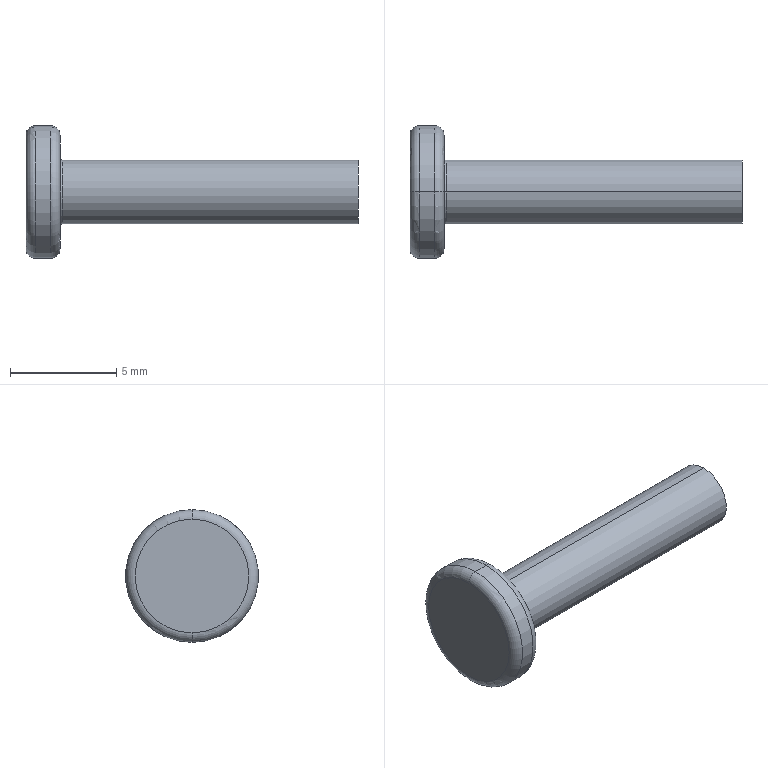Part | SolidWorks | features Revolution 1 | 1 solid | 13 faces | box 15.6 x 6.24 x 6.24 mm | volume 146.299 mm3 | torus 6 | cylinder 4 | plane 3 | commonest cylinder face diameters 3 x2 6.24 x2
STEP:
#1=CARTESIAN_POINT('',(0.4448,0.,3.12));
#2=VERTEX_POINT('',#1);
#3=CARTESIAN_POINT('',(0.4448,0.,-3.12));
#4=VERTEX_POINT('',#3);
#5=CARTESIAN_POINT('',(0.4448,0.,0.));
#6=DIRECTION('',(-1.,0.,0.));
#7=DIRECTION('',(0.,0.,1.));
#8=AXIS2_PLACEMENT_3D('',#5,#6,#7);
#9=CIRCLE('',#8,3.12);
#10=EDGE_CURVE('',#2,#4,#9,.T.);
#11=ORIENTED_EDGE('',*,*,#10,.T.);
#12=CARTESIAN_POINT('',(0.,0.,-2.675));
#13=VERTEX_POINT('',#12);
#14=CARTESIAN_POINT('',(0.4448,0.,-2.675));
#15=DIRECTION('',(0.,1.,0.));
#16=DIRECTION('',(0.,0.,1.));
#17=AXIS2_PLACEMENT_3D('',#14,#15,#16);
#18=CIRCLE('',#17,0.4448);
#19=EDGE_CURVE('',#4,#13,#18,.T.);
#20=ORIENTED_EDGE('',*,*,#19,.T.);
#21=CARTESIAN_POINT('',(0.,0.,2.675));
#22=VERTEX_POINT('',#21);
#23=CARTESIAN_POINT('',(0.,0.,0.));
#24=DIRECTION('',(-1.,0.,0.));
#25=DIRECTION('',(0.,0.,1.));
#26=AXIS2_PLACEMENT_3D('',#23,#24,#25);
#27=CIRCLE('',#26,2.675);
#28=EDGE_CURVE('',#22,#13,#27,.T.);
#29=ORIENTED_EDGE('',*,*,#28,.F.);
#30=CARTESIAN_POINT('',(0.4448,0.,2.675));
#31=DIRECTION('',(0.,-1.,0.));
#32=DIRECTION('',(0.,0.,-1.));
#33=AXIS2_PLACEMENT_3D('',#30,#31,#32);
#34=CIRCLE('',#33,0.4448);
#35=EDGE_CURVE('',#2,#22,#34,.T.);
#36=ORIENTED_EDGE('',*,*,#35,.F.);
#37=EDGE_LOOP('',(#11,#20,#29,#36));
#38=FACE_OUTER_BOUND('',#37,.T.);
#39=CARTESIAN_POINT('',(0.4448,0.,0.));
#40=DIRECTION('',(-1.,0.,0.));
#41=DIRECTION('',(0.,0.,1.));
#42=AXIS2_PLACEMENT_3D('',#39,#40,#41);
#43=TOROIDAL_SURFACE('',#42,2.675,0.4448);
#44=ADVANCED_FACE('',(#38),#43,.T.);
#45=CARTESIAN_POINT('',(1.155,0.,3.12));
#46=VERTEX_POINT('',#45);
#47=CARTESIAN_POINT('',(1.155,0.,-3.12));
#48=VERTEX_POINT('',#47);
#49=CARTESIAN_POINT('',(1.155,0.,0.));
#50=DIRECTION('',(-1.,0.,0.));
#51=DIRECTION('',(0.,0.,1.));
#52=AXIS2_PLACEMENT_3D('',#49,#50,#51);
#53=CIRCLE('',#52,3.12);
#54=EDGE_CURVE('',#46,#48,#53,.T.);
#55=ORIENTED_EDGE('',*,*,#54,.T.);
#56=CARTESIAN_POINT('',(0.,0.,-3.12));
#57=DIRECTION('',(-1.,0.,0.));
#58=VECTOR('',#57,1000.);
#59=LINE('',#56,#58);
#60=EDGE_CURVE('',#48,#4,#59,.T.);
#61=ORIENTED_EDGE('',*,*,#60,.T.);
#62=ORIENTED_EDGE('',*,*,#10,.F.);
#63=CARTESIAN_POINT('',(0.,0.,3.12));
#64=DIRECTION('',(-1.,0.,0.));
#65=VECTOR('',#64,1000.);
#66=LINE('',#63,#65);
#67=EDGE_CURVE('',#46,#2,#66,.T.);
#68=ORIENTED_EDGE('',*,*,#67,.F.);
#69=EDGE_LOOP('',(#55,#61,#62,#68));
#70=FACE_OUTER_BOUND('',#69,.T.);
#71=CARTESIAN_POINT('',(0.,0.,0.));
#72=DIRECTION('',(-1.,0.,0.));
#73=DIRECTION('',(0.,0.,1.));
#74=AXIS2_PLACEMENT_3D('',#71,#72,#73);
#75=CYLINDRICAL_SURFACE('',#74,3.12);
#76=ADVANCED_FACE('',(#70),#75,.T.);
#77=CARTESIAN_POINT('',(1.6,0.,2.675));
#78=VERTEX_POINT('',#77);
#79=CARTESIAN_POINT('',(1.6,0.,-2.675));
#80=VERTEX_POINT('',#79);
#81=CARTESIAN_POINT('',(1.6,0.,0.));
#82=DIRECTION('',(-1.,0.,0.));
#83=DIRECTION('',(0.,0.,1.));
#84=AXIS2_PLACEMENT_3D('',#81,#82,#83);
#85=CIRCLE('',#84,2.675);
#86=EDGE_CURVE('',#78,#80,#85,.T.);
#87=ORIENTED_EDGE('',*,*,#86,.T.);
#88=CARTESIAN_POINT('',(1.155,0.,-2.675));
#89=DIRECTION('',(0.,1.,0.));
#90=DIRECTION('',(0.,0.,1.));
#91=AXIS2_PLACEMENT_3D('',#88,#89,#90);
#92=CIRCLE('',#91,0.4448);
#93=EDGE_CURVE('',#80,#48,#92,.T.);
#94=ORIENTED_EDGE('',*,*,#93,.T.);
#95=ORIENTED_EDGE('',*,*,#54,.F.);
#96=CARTESIAN_POINT('',(1.155,0.,2.675));
#97=DIRECTION('',(0.,-1.,0.));
#98=DIRECTION('',(0.,0.,-1.));
#99=AXIS2_PLACEMENT_3D('',#96,#97,#98);
#100=CIRCLE('',#99,0.4448);
#101=EDGE_CURVE('',#78,#46,#100,.T.);
#102=ORIENTED_EDGE('',*,*,#101,.F.);
#103=EDGE_LOOP('',(#87,#94,#95,#102));
#104=FACE_OUTER_BOUND('',#103,.T.);
#105=CARTESIAN_POINT('',(1.155,0.,0.));
#106=DIRECTION('',(-1.,0.,0.));
#107=DIRECTION('',(0.,0.,1.));
#108=AXIS2_PLACEMENT_3D('',#105,#106,#107);
#109=TOROIDAL_SURFACE('',#108,2.675,0.4448);
#110=ADVANCED_FACE('',(#104),#109,.T.);
#111=CARTESIAN_POINT('',(1.6,0.,-1.6));
#112=VERTEX_POINT('',#111);
#113=CARTESIAN_POINT('',(1.6,0.,1.6));
#114=VERTEX_POINT('',#113);
#115=CARTESIAN_POINT('',(1.6,0.,0.));
#116=DIRECTION('',(-1.,0.,0.));
#117=DIRECTION('',(0.,0.,1.));
#118=AXIS2_PLACEMENT_3D('',#115,#116,#117);
#119=CIRCLE('',#118,1.6);
#120=EDGE_CURVE('',#112,#114,#119,.T.);
#121=ORIENTED_EDGE('',*,*,#120,.F.);
#122=CARTESIAN_POINT('',(1.7,0.,-1.5));
#123=VERTEX_POINT('',#122);
#124=CARTESIAN_POINT('',(1.7,0.,-1.6));
#125=DIRECTION('',(0.,1.,0.));
#126=DIRECTION('',(0.,0.,1.));
#127=AXIS2_PLACEMENT_3D('',#124,#125,#126);
#128=CIRCLE('',#127,0.1);
#129=EDGE_CURVE('',#112,#123,#128,.T.);
#130=ORIENTED_EDGE('',*,*,#129,.T.);
#131=CARTESIAN_POINT('',(1.7,0.,1.5));
#132=VERTEX_POINT('',#131);
#133=CARTESIAN_POINT('',(1.7,0.,0.));
#134=DIRECTION('',(-1.,0.,0.));
#135=DIRECTION('',(0.,0.,1.));
#136=AXIS2_PLACEMENT_3D('',#133,#134,#135);
#137=CIRCLE('',#136,1.5);
#138=EDGE_CURVE('',#123,#132,#137,.T.);
#139=ORIENTED_EDGE('',*,*,#138,.T.);
#140=CARTESIAN_POINT('',(1.7,0.,1.6));
#141=DIRECTION('',(0.,-1.,0.));
#142=DIRECTION('',(0.,0.,-1.));
#143=AXIS2_PLACEMENT_3D('',#140,#141,#142);
#144=CIRCLE('',#143,0.1);
#145=EDGE_CURVE('',#114,#132,#144,.T.);
#146=ORIENTED_EDGE('',*,*,#145,.F.);
#147=EDGE_LOOP('',(#121,#130,#139,#146));
#148=FACE_OUTER_BOUND('',#147,.T.);
#149=CARTESIAN_POINT('',(1.7,0.,0.));
#150=DIRECTION('',(-1.,0.,0.));
#151=DIRECTION('',(0.,0.,1.));
#152=AXIS2_PLACEMENT_3D('',#149,#150,#151);
#153=TOROIDAL_SURFACE('',#152,1.6,0.1);
#154=ADVANCED_FACE('',(#148),#153,.F.);
#155=CARTESIAN_POINT('',(15.6,0.,1.5));
#156=VERTEX_POINT('',#155);
#157=CARTESIAN_POINT('',(15.6,0.,-1.5));
#158=VERTEX_POINT('',#157);
#159=CARTESIAN_POINT('',(15.6,0.,0.));
#160=DIRECTION('',(-1.,0.,0.));
#161=DIRECTION('',(0.,0.,1.));
#162=AXIS2_PLACEMENT_3D('',#159,#160,#161);
#163=CIRCLE('',#162,1.5);
#164=EDGE_CURVE('',#156,#158,#163,.T.);
#165=ORIENTED_EDGE('',*,*,#164,.T.);
#166=CARTESIAN_POINT('',(0.,0.,-1.5));
#167=DIRECTION('',(-1.,0.,0.));
#168=VECTOR('',#167,1000.);
#169=LINE('',#166,#168);
#170=EDGE_CURVE('',#158,#123,#169,.T.);
#171=ORIENTED_EDGE('',*,*,#170,.T.);
#172=CARTESIAN_POINT('',(1.7,0.,0.));
#173=DIRECTION('',(-1.,0.,0.));
#174=DIRECTION('',(0.,0.,1.));
#175=AXIS2_PLACEMENT_3D('',#172,#173,#174);
#176=CIRCLE('',#175,1.5);
#177=EDGE_CURVE('',#132,#123,#176,.T.);
#178=ORIENTED_EDGE('',*,*,#177,.F.);
#179=CARTESIAN_POINT('',(0.,0.,1.5));
#180=DIRECTION('',(-1.,0.,0.));
#181=VECTOR('',#180,1000.);
#182=LINE('',#179,#181);
#183=EDGE_CURVE('',#156,#132,#182,.T.);
#184=ORIENTED_EDGE('',*,*,#183,.F.);
#185=EDGE_LOOP('',(#165,#171,#178,#184));
#186=FACE_OUTER_BOUND('',#185,.T.);
#187=CARTESIAN_POINT('',(0.,0.,0.));
#188=DIRECTION('',(-1.,0.,0.));
#189=DIRECTION('',(0.,0.,1.));
#190=AXIS2_PLACEMENT_3D('',#187,#188,#189);
#191=CYLINDRICAL_SURFACE('',#190,1.5);
#192=ADVANCED_FACE('',(#186),#191,.T.);
#193=ORIENTED_EDGE('',*,*,#164,.F.);
#194=CARTESIAN_POINT('',(15.6,0.,0.));
#195=DIRECTION('',(-1.,0.,0.));
#196=DIRECTION('',(0.,0.,1.));
#197=AXIS2_PLACEMENT_3D('',#194,#195,#196);
#198=CIRCLE('',#197,1.5);
#199=EDGE_CURVE('',#158,#156,#198,.T.);
#200=ORIENTED_EDGE('',*,*,#199,.F.);
#201=EDGE_LOOP('',(#193,#200));
#202=FACE_OUTER_BOUND('',#201,.T.);
#203=CARTESIAN_POINT('',(15.6,1.5,0.));
#204=DIRECTION('',(-1.,0.,0.));
#205=DIRECTION('',(0.,0.,1.));
#206=AXIS2_PLACEMENT_3D('',#203,#204,#205);
#207=PLANE('',#206);
#208=ADVANCED_FACE('',(#202),#207,.F.);
#209=ORIENTED_EDGE('',*,*,#170,.F.);
#210=ORIENTED_EDGE('',*,*,#199,.T.);
#211=ORIENTED_EDGE('',*,*,#183,.T.);
#212=ORIENTED_EDGE('',*,*,#138,.F.);
#213=EDGE_LOOP('',(#209,#210,#211,#212));
#214=FACE_OUTER_BOUND('',#213,.T.);
#215=CARTESIAN_POINT('',(0.,0.,0.));
#216=DIRECTION('',(-1.,0.,0.));
#217=DIRECTION('',(0.,0.,1.));
#218=AXIS2_PLACEMENT_3D('',#215,#216,#217);
#219=CYLINDRICAL_SURFACE('',#218,1.5);
#220=ADVANCED_FACE('',(#214),#219,.T.);
#221=ORIENTED_EDGE('',*,*,#129,.F.);
#222=CARTESIAN_POINT('',(1.6,0.,0.));
#223=DIRECTION('',(-1.,0.,0.));
#224=DIRECTION('',(0.,0.,1.));
#225=AXIS2_PLACEMENT_3D('',#222,#223,#224);
#226=CIRCLE('',#225,1.6);
#227=EDGE_CURVE('',#114,#112,#226,.T.);
#228=ORIENTED_EDGE('',*,*,#227,.F.);
#229=ORIENTED_EDGE('',*,*,#145,.T.);
#230=ORIENTED_EDGE('',*,*,#177,.T.);
#231=EDGE_LOOP('',(#221,#228,#229,#230));
#232=FACE_OUTER_BOUND('',#231,.T.);
#233=CARTESIAN_POINT('',(1.7,0.,0.));
#234=DIRECTION('',(-1.,0.,0.));
#235=DIRECTION('',(0.,0.,1.));
#236=AXIS2_PLACEMENT_3D('',#233,#234,#235);
#237=TOROIDAL_SURFACE('',#236,1.6,0.1);
#238=ADVANCED_FACE('',(#232),#237,.F.);
#239=ORIENTED_EDGE('',*,*,#86,.F.);
#240=CARTESIAN_POINT('',(1.6,0.,0.));
#241=DIRECTION('',(-1.,0.,0.));
#242=DIRECTION('',(0.,0.,1.));
#243=AXIS2_PLACEMENT_3D('',#240,#241,#242);
#244=CIRCLE('',#243,2.675);
#245=EDGE_CURVE('',#80,#78,#244,.T.);
#246=ORIENTED_EDGE('',*,*,#245,.F.);
#247=EDGE_LOOP('',(#239,#246));
#248=FACE_OUTER_BOUND('',#247,.T.);
#249=ORIENTED_EDGE('',*,*,#227,.T.);
#250=ORIENTED_EDGE('',*,*,#120,.T.);
#251=EDGE_LOOP('',(#249,#250));
#252=FACE_BOUND('',#251,.T.);
#253=CARTESIAN_POINT('',(1.6,2.675,0.));
#254=DIRECTION('',(-1.,0.,0.));
#255=DIRECTION('',(0.,0.,1.));
#256=AXIS2_PLACEMENT_3D('',#253,#254,#255);
#257=PLANE('',#256);
#258=ADVANCED_FACE('',(#248,#252),#257,.F.);
#259=ORIENTED_EDGE('',*,*,#93,.F.);
#260=ORIENTED_EDGE('',*,*,#245,.T.);
#261=ORIENTED_EDGE('',*,*,#101,.T.);
#262=CARTESIAN_POINT('',(1.155,0.,0.));
#263=DIRECTION('',(-1.,0.,0.));
#264=DIRECTION('',(0.,0.,1.));
#265=AXIS2_PLACEMENT_3D('',#262,#263,#264);
#266=CIRCLE('',#265,3.12);
#267=EDGE_CURVE('',#48,#46,#266,.T.);
#268=ORIENTED_EDGE('',*,*,#267,.F.);
#269=EDGE_LOOP('',(#259,#260,#261,#268));
#270=FACE_OUTER_BOUND('',#269,.T.);
#271=CARTESIAN_POINT('',(1.155,0.,0.));
#272=DIRECTION('',(-1.,0.,0.));
#273=DIRECTION('',(0.,0.,1.));
#274=AXIS2_PLACEMENT_3D('',#271,#272,#273);
#275=TOROIDAL_SURFACE('',#274,2.675,0.4448);
#276=ADVANCED_FACE('',(#270),#275,.T.);
#277=ORIENTED_EDGE('',*,*,#60,.F.);
#278=ORIENTED_EDGE('',*,*,#267,.T.);
#279=ORIENTED_EDGE('',*,*,#67,.T.);
#280=CARTESIAN_POINT('',(0.4448,0.,0.));
#281=DIRECTION('',(-1.,0.,0.));
#282=DIRECTION('',(0.,0.,1.));
#283=AXIS2_PLACEMENT_3D('',#280,#281,#282);
#284=CIRCLE('',#283,3.12);
#285=EDGE_CURVE('',#4,#2,#284,.T.);
#286=ORIENTED_EDGE('',*,*,#285,.F.);
#287=EDGE_LOOP('',(#277,#278,#279,#286));
#288=FACE_OUTER_BOUND('',#287,.T.);
#289=CARTESIAN_POINT('',(0.,0.,0.));
#290=DIRECTION('',(-1.,0.,0.));
#291=DIRECTION('',(0.,0.,1.));
#292=AXIS2_PLACEMENT_3D('',#289,#290,#291);
#293=CYLINDRICAL_SURFACE('',#292,3.12);
#294=ADVANCED_FACE('',(#288),#293,.T.);
#295=ORIENTED_EDGE('',*,*,#19,.F.);
#296=ORIENTED_EDGE('',*,*,#285,.T.);
#297=ORIENTED_EDGE('',*,*,#35,.T.);
#298=CARTESIAN_POINT('',(0.,0.,0.));
#299=DIRECTION('',(-1.,0.,0.));
#300=DIRECTION('',(0.,0.,1.));
#301=AXIS2_PLACEMENT_3D('',#298,#299,#300);
#302=CIRCLE('',#301,2.675);
#303=EDGE_CURVE('',#13,#22,#302,.T.);
#304=ORIENTED_EDGE('',*,*,#303,.F.);
#305=EDGE_LOOP('',(#295,#296,#297,#304));
#306=FACE_OUTER_BOUND('',#305,.T.);
#307=CARTESIAN_POINT('',(0.4448,0.,0.));
#308=DIRECTION('',(-1.,0.,0.));
#309=DIRECTION('',(0.,0.,1.));
#310=AXIS2_PLACEMENT_3D('',#307,#308,#309);
#311=TOROIDAL_SURFACE('',#310,2.675,0.4448);
#312=ADVANCED_FACE('',(#306),#311,.T.);
#313=ORIENTED_EDGE('',*,*,#28,.T.);
#314=ORIENTED_EDGE('',*,*,#303,.T.);
#315=EDGE_LOOP('',(#313,#314));
#316=FACE_OUTER_BOUND('',#315,.T.);
#317=CARTESIAN_POINT('',(0.,0.,0.));
#318=DIRECTION('',(1.,0.,0.));
#319=DIRECTION('',(0.,0.,-1.));
#320=AXIS2_PLACEMENT_3D('',#317,#318,#319);
#321=PLANE('',#320);
#322=ADVANCED_FACE('',(#316),#321,.F.);
#323=CLOSED_SHELL('',(#44,#76,#110,#154,#192,#208,#220,#238,#258,#276,#294,#312,#322));
#324=MANIFOLD_SOLID_BREP('',#323);
#325=CARTESIAN_POINT('',(0.,0.,0.));
#326=DIRECTION('',(0.,0.,1.));
#327=DIRECTION('',(1.,0.,0.));
#328=AXIS2_PLACEMENT_3D('',#325,#326,#327);
#329=(LENGTH_UNIT()NAMED_UNIT(*)SI_UNIT(.MILLI.,.METRE.));
#330=UNCERTAINTY_MEASURE_WITH_UNIT(LENGTH_MEASURE(0.00001),#329,'','');
#331=(NAMED_UNIT(*)PLANE_ANGLE_UNIT()SI_UNIT($,.RADIAN.));
#332=(NAMED_UNIT(*)SI_UNIT($,.STERADIAN.)SOLID_ANGLE_UNIT());
#333=(GEOMETRIC_REPRESENTATION_CONTEXT(3)GLOBAL_UNCERTAINTY_ASSIGNED_CONTEXT((#330))GLOBAL_UNIT_ASSIGNED_CONTEXT((#329,#331,#332))REPRESENTATION_CONTEXT('',''));
#334=ADVANCED_BREP_SHAPE_REPRESENTATION('',(#324,#328),#333);